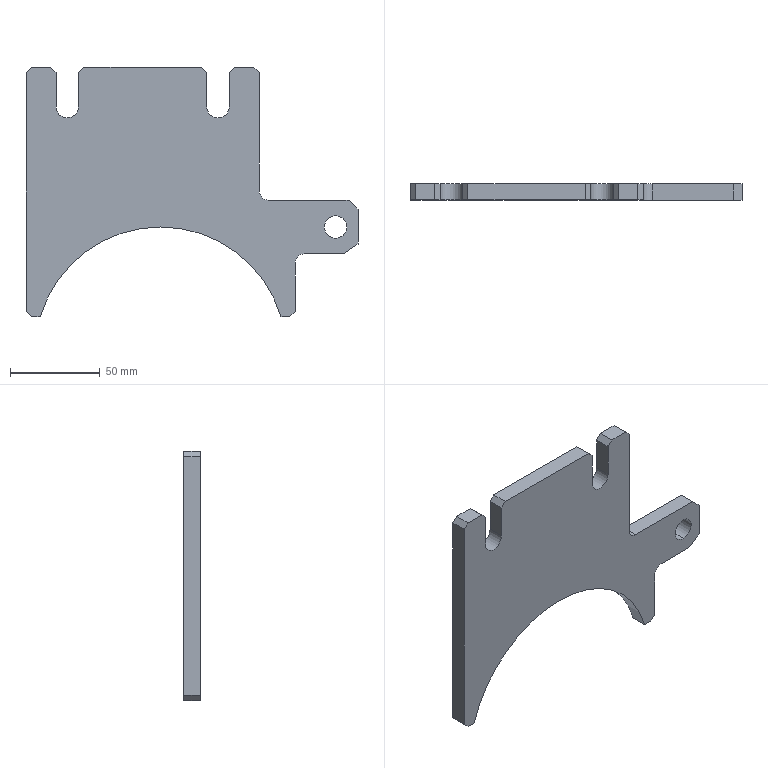Part | SolidWorks | features FlatPattern 1, SMBaseFlange 1, SheetMetal 1 | 1 solid | 35 faces | box 185 x 9 x 139 mm | volume 131664 mm3 | plane 27 | cylinder 8 | commonest cylinder face diameters 12.5 x4 10 x2 140 x2
STEP:
#1=CARTESIAN_POINT('',(172.5,-9.,43.75));
#2=VERTEX_POINT('',#1);
#3=CARTESIAN_POINT('',(172.5,-9.,56.25));
#4=VERTEX_POINT('',#3);
#5=CARTESIAN_POINT('',(172.5,-9.,50.));
#6=DIRECTION('',(0.,1.,0.));
#7=DIRECTION('',(0.,0.,1.));
#8=AXIS2_PLACEMENT_3D('',#5,#6,#7);
#9=CIRCLE('',#8,6.25);
#10=EDGE_CURVE('',#2,#4,#9,.T.);
#11=ORIENTED_EDGE('',*,*,#10,.F.);
#12=CARTESIAN_POINT('',(172.5,0.,43.75));
#13=VERTEX_POINT('',#12);
#14=CARTESIAN_POINT('',(172.5,-9.,43.75));
#15=DIRECTION('',(0.,1.,0.));
#16=VECTOR('',#15,1000.);
#17=LINE('',#14,#16);
#18=EDGE_CURVE('',#2,#13,#17,.T.);
#19=ORIENTED_EDGE('',*,*,#18,.T.);
#20=CARTESIAN_POINT('',(172.5,0.,56.25));
#21=VERTEX_POINT('',#20);
#22=CARTESIAN_POINT('',(172.5,0.,50.));
#23=DIRECTION('',(0.,1.,0.));
#24=DIRECTION('',(0.,0.,1.));
#25=AXIS2_PLACEMENT_3D('',#22,#23,#24);
#26=CIRCLE('',#25,6.25);
#27=EDGE_CURVE('',#13,#21,#26,.T.);
#28=ORIENTED_EDGE('',*,*,#27,.T.);
#29=CARTESIAN_POINT('',(172.5,-9.,56.25));
#30=DIRECTION('',(0.,1.,0.));
#31=VECTOR('',#30,1000.);
#32=LINE('',#29,#31);
#33=EDGE_CURVE('',#4,#21,#32,.T.);
#34=ORIENTED_EDGE('',*,*,#33,.F.);
#35=EDGE_LOOP('',(#11,#19,#28,#34));
#36=FACE_OUTER_BOUND('',#35,.T.);
#37=CARTESIAN_POINT('',(172.5,-9.,50.));
#38=DIRECTION('',(0.,1.,0.));
#39=DIRECTION('',(0.,0.,1.));
#40=AXIS2_PLACEMENT_3D('',#37,#38,#39);
#41=CYLINDRICAL_SURFACE('',#40,6.25);
#42=ADVANCED_FACE('',(#36),#41,.F.);
#43=CARTESIAN_POINT('',(142.082,-9.,0.));
#44=VERTEX_POINT('',#43);
#45=CARTESIAN_POINT('',(75.,-9.,50.));
#46=VERTEX_POINT('',#45);
#47=CARTESIAN_POINT('',(75.,-9.,-20.));
#48=DIRECTION('',(0.,-1.,0.));
#49=DIRECTION('',(0.,0.,1.));
#50=AXIS2_PLACEMENT_3D('',#47,#48,#49);
#51=CIRCLE('',#50,70.);
#52=EDGE_CURVE('',#44,#46,#51,.T.);
#53=ORIENTED_EDGE('',*,*,#52,.T.);
#54=CARTESIAN_POINT('',(75.,0.,50.));
#55=VERTEX_POINT('',#54);
#56=CARTESIAN_POINT('',(75.,-9.,50.));
#57=DIRECTION('',(0.,1.,0.));
#58=VECTOR('',#57,1000.);
#59=LINE('',#56,#58);
#60=EDGE_CURVE('',#46,#55,#59,.T.);
#61=ORIENTED_EDGE('',*,*,#60,.T.);
#62=CARTESIAN_POINT('',(142.082,0.,0.));
#63=VERTEX_POINT('',#62);
#64=CARTESIAN_POINT('',(75.,0.,-20.));
#65=DIRECTION('',(0.,-1.,0.));
#66=DIRECTION('',(0.,0.,1.));
#67=AXIS2_PLACEMENT_3D('',#64,#65,#66);
#68=CIRCLE('',#67,70.);
#69=EDGE_CURVE('',#63,#55,#68,.T.);
#70=ORIENTED_EDGE('',*,*,#69,.F.);
#71=CARTESIAN_POINT('',(142.082,-9.,0.));
#72=DIRECTION('',(0.,1.,0.));
#73=VECTOR('',#72,1000.);
#74=LINE('',#71,#73);
#75=EDGE_CURVE('',#44,#63,#74,.T.);
#76=ORIENTED_EDGE('',*,*,#75,.F.);
#77=EDGE_LOOP('',(#53,#61,#70,#76));
#78=FACE_OUTER_BOUND('',#77,.T.);
#79=CARTESIAN_POINT('',(75.,-9.,-20.));
#80=DIRECTION('',(0.,1.,0.));
#81=DIRECTION('',(0.,0.,1.));
#82=AXIS2_PLACEMENT_3D('',#79,#80,#81);
#83=CYLINDRICAL_SURFACE('',#82,70.);
#84=ADVANCED_FACE('',(#78),#83,.F.);
#85=ORIENTED_EDGE('',*,*,#60,.F.);
#86=CARTESIAN_POINT('',(7.918,-9.,0.));
#87=VERTEX_POINT('',#86);
#88=CARTESIAN_POINT('',(75.,-9.,-20.));
#89=DIRECTION('',(0.,-1.,0.));
#90=DIRECTION('',(0.,0.,1.));
#91=AXIS2_PLACEMENT_3D('',#88,#89,#90);
#92=CIRCLE('',#91,70.);
#93=EDGE_CURVE('',#46,#87,#92,.T.);
#94=ORIENTED_EDGE('',*,*,#93,.T.);
#95=CARTESIAN_POINT('',(7.918,0.,0.));
#96=VERTEX_POINT('',#95);
#97=CARTESIAN_POINT('',(7.918,-9.,0.));
#98=DIRECTION('',(0.,1.,0.));
#99=VECTOR('',#98,1000.);
#100=LINE('',#97,#99);
#101=EDGE_CURVE('',#87,#96,#100,.T.);
#102=ORIENTED_EDGE('',*,*,#101,.T.);
#103=CARTESIAN_POINT('',(75.,0.,-20.));
#104=DIRECTION('',(0.,-1.,0.));
#105=DIRECTION('',(0.,0.,1.));
#106=AXIS2_PLACEMENT_3D('',#103,#104,#105);
#107=CIRCLE('',#106,70.);
#108=EDGE_CURVE('',#55,#96,#107,.T.);
#109=ORIENTED_EDGE('',*,*,#108,.F.);
#110=EDGE_LOOP('',(#85,#94,#102,#109));
#111=FACE_OUTER_BOUND('',#110,.T.);
#112=CARTESIAN_POINT('',(75.,-9.,-20.));
#113=DIRECTION('',(0.,1.,0.));
#114=DIRECTION('',(0.,0.,1.));
#115=AXIS2_PLACEMENT_3D('',#112,#113,#114);
#116=CYLINDRICAL_SURFACE('',#115,70.);
#117=ADVANCED_FACE('',(#111),#116,.F.);
#118=CARTESIAN_POINT('',(147.,0.,0.));
#119=VERTEX_POINT('',#118);
#120=CARTESIAN_POINT('',(142.082,0.,0.));
#121=DIRECTION('',(-1.,0.,0.));
#122=VECTOR('',#121,1000.);
#123=LINE('',#120,#122);
#124=EDGE_CURVE('',#119,#63,#123,.T.);
#125=ORIENTED_EDGE('',*,*,#124,.F.);
#126=CARTESIAN_POINT('',(147.,-9.,0.));
#127=VERTEX_POINT('',#126);
#128=CARTESIAN_POINT('',(147.,-9.,0.));
#129=DIRECTION('',(0.,1.,0.));
#130=VECTOR('',#129,1000.);
#131=LINE('',#128,#130);
#132=EDGE_CURVE('',#127,#119,#131,.T.);
#133=ORIENTED_EDGE('',*,*,#132,.F.);
#134=CARTESIAN_POINT('',(142.082,-9.,0.));
#135=DIRECTION('',(-1.,0.,0.));
#136=VECTOR('',#135,1000.);
#137=LINE('',#134,#136);
#138=EDGE_CURVE('',#127,#44,#137,.T.);
#139=ORIENTED_EDGE('',*,*,#138,.T.);
#140=ORIENTED_EDGE('',*,*,#75,.T.);
#141=EDGE_LOOP('',(#125,#133,#139,#140));
#142=FACE_OUTER_BOUND('',#141,.T.);
#143=CARTESIAN_POINT('',(142.082,-9.,0.));
#144=DIRECTION('',(0.,0.,-1.));
#145=DIRECTION('',(-1.,0.,0.));
#146=AXIS2_PLACEMENT_3D('',#143,#144,#145);
#147=PLANE('',#146);
#148=ADVANCED_FACE('',(#142),#147,.T.);
#149=CARTESIAN_POINT('',(150.,0.,3.));
#150=VERTEX_POINT('',#149);
#151=CARTESIAN_POINT('',(147.,0.,0.));
#152=DIRECTION('',(-0.7071,0.,-0.7071));
#153=VECTOR('',#152,1000.);
#154=LINE('',#151,#153);
#155=EDGE_CURVE('',#150,#119,#154,.T.);
#156=ORIENTED_EDGE('',*,*,#155,.F.);
#157=CARTESIAN_POINT('',(150.,-9.,3.));
#158=VERTEX_POINT('',#157);
#159=CARTESIAN_POINT('',(150.,-9.,3.));
#160=DIRECTION('',(0.,1.,0.));
#161=VECTOR('',#160,1000.);
#162=LINE('',#159,#161);
#163=EDGE_CURVE('',#158,#150,#162,.T.);
#164=ORIENTED_EDGE('',*,*,#163,.F.);
#165=CARTESIAN_POINT('',(147.,-9.,0.));
#166=DIRECTION('',(-0.7071,0.,-0.7071));
#167=VECTOR('',#166,1000.);
#168=LINE('',#165,#167);
#169=EDGE_CURVE('',#158,#127,#168,.T.);
#170=ORIENTED_EDGE('',*,*,#169,.T.);
#171=ORIENTED_EDGE('',*,*,#132,.T.);
#172=EDGE_LOOP('',(#156,#164,#170,#171));
#173=FACE_OUTER_BOUND('',#172,.T.);
#174=CARTESIAN_POINT('',(147.,-9.,0.));
#175=DIRECTION('',(0.7071,0.,-0.7071));
#176=DIRECTION('',(-0.7071,0.,-0.7071));
#177=AXIS2_PLACEMENT_3D('',#174,#175,#176);
#178=PLANE('',#177);
#179=ADVANCED_FACE('',(#173),#178,.T.);
#180=CARTESIAN_POINT('',(150.,0.,30.));
#181=VERTEX_POINT('',#180);
#182=CARTESIAN_POINT('',(150.,0.,3.));
#183=DIRECTION('',(0.,0.,-1.));
#184=VECTOR('',#183,1000.);
#185=LINE('',#182,#184);
#186=EDGE_CURVE('',#181,#150,#185,.T.);
#187=ORIENTED_EDGE('',*,*,#186,.F.);
#188=CARTESIAN_POINT('',(150.,-9.,30.));
#189=VERTEX_POINT('',#188);
#190=CARTESIAN_POINT('',(150.,-9.,30.));
#191=DIRECTION('',(0.,1.,0.));
#192=VECTOR('',#191,1000.);
#193=LINE('',#190,#192);
#194=EDGE_CURVE('',#189,#181,#193,.T.);
#195=ORIENTED_EDGE('',*,*,#194,.F.);
#196=CARTESIAN_POINT('',(150.,-9.,3.));
#197=DIRECTION('',(0.,0.,-1.));
#198=VECTOR('',#197,1000.);
#199=LINE('',#196,#198);
#200=EDGE_CURVE('',#189,#158,#199,.T.);
#201=ORIENTED_EDGE('',*,*,#200,.T.);
#202=ORIENTED_EDGE('',*,*,#163,.T.);
#203=EDGE_LOOP('',(#187,#195,#201,#202));
#204=FACE_OUTER_BOUND('',#203,.T.);
#205=CARTESIAN_POINT('',(150.,-9.,3.));
#206=DIRECTION('',(1.,0.,0.));
#207=DIRECTION('',(0.,0.,-1.));
#208=AXIS2_PLACEMENT_3D('',#205,#206,#207);
#209=PLANE('',#208);
#210=ADVANCED_FACE('',(#204),#209,.T.);
#211=CARTESIAN_POINT('',(155.,0.,35.));
#212=VERTEX_POINT('',#211);
#213=CARTESIAN_POINT('',(155.,0.,30.));
#214=DIRECTION('',(0.,-1.,0.));
#215=DIRECTION('',(0.,0.,1.));
#216=AXIS2_PLACEMENT_3D('',#213,#214,#215);
#217=CIRCLE('',#216,5.);
#218=EDGE_CURVE('',#212,#181,#217,.T.);
#219=ORIENTED_EDGE('',*,*,#218,.F.);
#220=CARTESIAN_POINT('',(155.,-9.,35.));
#221=VERTEX_POINT('',#220);
#222=CARTESIAN_POINT('',(155.,-9.,35.));
#223=DIRECTION('',(0.,1.,0.));
#224=VECTOR('',#223,1000.);
#225=LINE('',#222,#224);
#226=EDGE_CURVE('',#221,#212,#225,.T.);
#227=ORIENTED_EDGE('',*,*,#226,.F.);
#228=CARTESIAN_POINT('',(155.,-9.,30.));
#229=DIRECTION('',(0.,-1.,0.));
#230=DIRECTION('',(0.,0.,1.));
#231=AXIS2_PLACEMENT_3D('',#228,#229,#230);
#232=CIRCLE('',#231,5.);
#233=EDGE_CURVE('',#221,#189,#232,.T.);
#234=ORIENTED_EDGE('',*,*,#233,.T.);
#235=ORIENTED_EDGE('',*,*,#194,.T.);
#236=EDGE_LOOP('',(#219,#227,#234,#235));
#237=FACE_OUTER_BOUND('',#236,.T.);
#238=CARTESIAN_POINT('',(155.,-9.,30.));
#239=DIRECTION('',(0.,1.,0.));
#240=DIRECTION('',(0.,0.,1.));
#241=AXIS2_PLACEMENT_3D('',#238,#239,#240);
#242=CYLINDRICAL_SURFACE('',#241,5.);
#243=ADVANCED_FACE('',(#237),#242,.F.);
#244=CARTESIAN_POINT('',(177.,0.,35.));
#245=VERTEX_POINT('',#244);
#246=CARTESIAN_POINT('',(155.,0.,35.));
#247=DIRECTION('',(-1.,0.,0.));
#248=VECTOR('',#247,1000.);
#249=LINE('',#246,#248);
#250=EDGE_CURVE('',#245,#212,#249,.T.);
#251=ORIENTED_EDGE('',*,*,#250,.F.);
#252=CARTESIAN_POINT('',(177.,-9.,35.));
#253=VERTEX_POINT('',#252);
#254=CARTESIAN_POINT('',(177.,-9.,35.));
#255=DIRECTION('',(0.,1.,0.));
#256=VECTOR('',#255,1000.);
#257=LINE('',#254,#256);
#258=EDGE_CURVE('',#253,#245,#257,.T.);
#259=ORIENTED_EDGE('',*,*,#258,.F.);
#260=CARTESIAN_POINT('',(155.,-9.,35.));
#261=DIRECTION('',(-1.,0.,0.));
#262=VECTOR('',#261,1000.);
#263=LINE('',#260,#262);
#264=EDGE_CURVE('',#253,#221,#263,.T.);
#265=ORIENTED_EDGE('',*,*,#264,.T.);
#266=ORIENTED_EDGE('',*,*,#226,.T.);
#267=EDGE_LOOP('',(#251,#259,#265,#266));
#268=FACE_OUTER_BOUND('',#267,.T.);
#269=CARTESIAN_POINT('',(155.,-9.,35.));
#270=DIRECTION('',(0.,0.,-1.));
#271=DIRECTION('',(-1.,0.,0.));
#272=AXIS2_PLACEMENT_3D('',#269,#270,#271);
#273=PLANE('',#272);
#274=ADVANCED_FACE('',(#268),#273,.T.);
#275=CARTESIAN_POINT('',(185.,0.,40.5));
#276=VERTEX_POINT('',#275);
#277=CARTESIAN_POINT('',(185.,0.,40.5));
#278=DIRECTION('',(-0.824,0.,-0.5665));
#279=VECTOR('',#278,1000.);
#280=LINE('',#277,#279);
#281=EDGE_CURVE('',#276,#245,#280,.T.);
#282=ORIENTED_EDGE('',*,*,#281,.F.);
#283=CARTESIAN_POINT('',(185.,-9.,40.5));
#284=VERTEX_POINT('',#283);
#285=CARTESIAN_POINT('',(185.,-9.,40.5));
#286=DIRECTION('',(0.,1.,0.));
#287=VECTOR('',#286,1000.);
#288=LINE('',#285,#287);
#289=EDGE_CURVE('',#284,#276,#288,.T.);
#290=ORIENTED_EDGE('',*,*,#289,.F.);
#291=CARTESIAN_POINT('',(185.,-9.,40.5));
#292=DIRECTION('',(-0.824,0.,-0.5665));
#293=VECTOR('',#292,1000.);
#294=LINE('',#291,#293);
#295=EDGE_CURVE('',#284,#253,#294,.T.);
#296=ORIENTED_EDGE('',*,*,#295,.T.);
#297=ORIENTED_EDGE('',*,*,#258,.T.);
#298=EDGE_LOOP('',(#282,#290,#296,#297));
#299=FACE_OUTER_BOUND('',#298,.T.);
#300=CARTESIAN_POINT('',(185.,-9.,40.5));
#301=DIRECTION('',(0.5665,0.,-0.824));
#302=DIRECTION('',(-0.824,0.,-0.5665));
#303=AXIS2_PLACEMENT_3D('',#300,#301,#302);
#304=PLANE('',#303);
#305=ADVANCED_FACE('',(#299),#304,.T.);
#306=CARTESIAN_POINT('',(185.,0.,60.));
#307=VERTEX_POINT('',#306);
#308=CARTESIAN_POINT('',(185.,0.,40.5));
#309=DIRECTION('',(0.,0.,-1.));
#310=VECTOR('',#309,1000.);
#311=LINE('',#308,#310);
#312=EDGE_CURVE('',#307,#276,#311,.T.);
#313=ORIENTED_EDGE('',*,*,#312,.F.);
#314=CARTESIAN_POINT('',(185.,-9.,60.));
#315=VERTEX_POINT('',#314);
#316=CARTESIAN_POINT('',(185.,-9.,60.));
#317=DIRECTION('',(0.,1.,0.));
#318=VECTOR('',#317,1000.);
#319=LINE('',#316,#318);
#320=EDGE_CURVE('',#315,#307,#319,.T.);
#321=ORIENTED_EDGE('',*,*,#320,.F.);
#322=CARTESIAN_POINT('',(185.,-9.,40.5));
#323=DIRECTION('',(0.,0.,-1.));
#324=VECTOR('',#323,1000.);
#325=LINE('',#322,#324);
#326=EDGE_CURVE('',#315,#284,#325,.T.);
#327=ORIENTED_EDGE('',*,*,#326,.T.);
#328=ORIENTED_EDGE('',*,*,#289,.T.);
#329=EDGE_LOOP('',(#313,#321,#327,#328));
#330=FACE_OUTER_BOUND('',#329,.T.);
#331=CARTESIAN_POINT('',(185.,-9.,40.5));
#332=DIRECTION('',(1.,0.,0.));
#333=DIRECTION('',(0.,0.,-1.));
#334=AXIS2_PLACEMENT_3D('',#331,#332,#333);
#335=PLANE('',#334);
#336=ADVANCED_FACE('',(#330),#335,.T.);
#337=CARTESIAN_POINT('',(180.,0.,65.));
#338=VERTEX_POINT('',#337);
#339=CARTESIAN_POINT('',(185.,0.,60.));
#340=DIRECTION('',(0.7071,0.,-0.7071));
#341=VECTOR('',#340,1000.);
#342=LINE('',#339,#341);
#343=EDGE_CURVE('',#338,#307,#342,.T.);
#344=ORIENTED_EDGE('',*,*,#343,.F.);
#345=CARTESIAN_POINT('',(180.,-9.,65.));
#346=VERTEX_POINT('',#345);
#347=CARTESIAN_POINT('',(180.,-9.,65.));
#348=DIRECTION('',(0.,1.,0.));
#349=VECTOR('',#348,1000.);
#350=LINE('',#347,#349);
#351=EDGE_CURVE('',#346,#338,#350,.T.);
#352=ORIENTED_EDGE('',*,*,#351,.F.);
#353=CARTESIAN_POINT('',(185.,-9.,60.));
#354=DIRECTION('',(0.7071,0.,-0.7071));
#355=VECTOR('',#354,1000.);
#356=LINE('',#353,#355);
#357=EDGE_CURVE('',#346,#315,#356,.T.);
#358=ORIENTED_EDGE('',*,*,#357,.T.);
#359=ORIENTED_EDGE('',*,*,#320,.T.);
#360=EDGE_LOOP('',(#344,#352,#358,#359));
#361=FACE_OUTER_BOUND('',#360,.T.);
#362=CARTESIAN_POINT('',(185.,-9.,60.));
#363=DIRECTION('',(0.7071,0.,0.7071));
#364=DIRECTION('',(0.7071,0.,-0.7071));
#365=AXIS2_PLACEMENT_3D('',#362,#363,#364);
#366=PLANE('',#365);
#367=ADVANCED_FACE('',(#361),#366,.T.);
#368=CARTESIAN_POINT('',(135.,0.,65.));
#369=VERTEX_POINT('',#368);
#370=CARTESIAN_POINT('',(180.,0.,65.));
#371=DIRECTION('',(1.,0.,0.));
#372=VECTOR('',#371,1000.);
#373=LINE('',#370,#372);
#374=EDGE_CURVE('',#369,#338,#373,.T.);
#375=ORIENTED_EDGE('',*,*,#374,.F.);
#376=CARTESIAN_POINT('',(135.,-9.,65.));
#377=VERTEX_POINT('',#376);
#378=CARTESIAN_POINT('',(135.,-9.,65.));
#379=DIRECTION('',(0.,1.,0.));
#380=VECTOR('',#379,1000.);
#381=LINE('',#378,#380);
#382=EDGE_CURVE('',#377,#369,#381,.T.);
#383=ORIENTED_EDGE('',*,*,#382,.F.);
#384=CARTESIAN_POINT('',(180.,-9.,65.));
#385=DIRECTION('',(1.,0.,0.));
#386=VECTOR('',#385,1000.);
#387=LINE('',#384,#386);
#388=EDGE_CURVE('',#377,#346,#387,.T.);
#389=ORIENTED_EDGE('',*,*,#388,.T.);
#390=ORIENTED_EDGE('',*,*,#351,.T.);
#391=EDGE_LOOP('',(#375,#383,#389,#390));
#392=FACE_OUTER_BOUND('',#391,.T.);
#393=CARTESIAN_POINT('',(180.,-9.,65.));
#394=DIRECTION('',(0.,0.,1.));
#395=DIRECTION('',(1.,0.,0.));
#396=AXIS2_PLACEMENT_3D('',#393,#394,#395);
#397=PLANE('',#396);
#398=ADVANCED_FACE('',(#392),#397,.T.);
#399=CARTESIAN_POINT('',(130.,0.,70.));
#400=VERTEX_POINT('',#399);
#401=CARTESIAN_POINT('',(135.,0.,70.));
#402=DIRECTION('',(0.,-1.,0.));
#403=DIRECTION('',(0.,0.,1.));
#404=AXIS2_PLACEMENT_3D('',#401,#402,#403);
#405=CIRCLE('',#404,5.);
#406=EDGE_CURVE('',#400,#369,#405,.T.);
#407=ORIENTED_EDGE('',*,*,#406,.F.);
#408=CARTESIAN_POINT('',(130.,-9.,70.));
#409=VERTEX_POINT('',#408);
#410=CARTESIAN_POINT('',(130.,-9.,70.));
#411=DIRECTION('',(0.,1.,0.));
#412=VECTOR('',#411,1000.);
#413=LINE('',#410,#412);
#414=EDGE_CURVE('',#409,#400,#413,.T.);
#415=ORIENTED_EDGE('',*,*,#414,.F.);
#416=CARTESIAN_POINT('',(135.,-9.,70.));
#417=DIRECTION('',(0.,-1.,0.));
#418=DIRECTION('',(0.,0.,1.));
#419=AXIS2_PLACEMENT_3D('',#416,#417,#418);
#420=CIRCLE('',#419,5.);
#421=EDGE_CURVE('',#409,#377,#420,.T.);
#422=ORIENTED_EDGE('',*,*,#421,.T.);
#423=ORIENTED_EDGE('',*,*,#382,.T.);
#424=EDGE_LOOP('',(#407,#415,#422,#423));
#425=FACE_OUTER_BOUND('',#424,.T.);
#426=CARTESIAN_POINT('',(135.,-9.,70.));
#427=DIRECTION('',(0.,1.,0.));
#428=DIRECTION('',(0.,0.,1.));
#429=AXIS2_PLACEMENT_3D('',#426,#427,#428);
#430=CYLINDRICAL_SURFACE('',#429,5.);
#431=ADVANCED_FACE('',(#425),#430,.F.);
#432=CARTESIAN_POINT('',(130.,0.,136.));
#433=VERTEX_POINT('',#432);
#434=CARTESIAN_POINT('',(130.,0.,70.));
#435=DIRECTION('',(0.,0.,-1.));
#436=VECTOR('',#435,1000.);
#437=LINE('',#434,#436);
#438=EDGE_CURVE('',#433,#400,#437,.T.);
#439=ORIENTED_EDGE('',*,*,#438,.F.);
#440=CARTESIAN_POINT('',(130.,-9.,136.));
#441=VERTEX_POINT('',#440);
#442=CARTESIAN_POINT('',(130.,-9.,136.));
#443=DIRECTION('',(0.,1.,0.));
#444=VECTOR('',#443,1000.);
#445=LINE('',#442,#444);
#446=EDGE_CURVE('',#441,#433,#445,.T.);
#447=ORIENTED_EDGE('',*,*,#446,.F.);
#448=CARTESIAN_POINT('',(130.,-9.,70.));
#449=DIRECTION('',(0.,0.,-1.));
#450=VECTOR('',#449,1000.);
#451=LINE('',#448,#450);
#452=EDGE_CURVE('',#441,#409,#451,.T.);
#453=ORIENTED_EDGE('',*,*,#452,.T.);
#454=ORIENTED_EDGE('',*,*,#414,.T.);
#455=EDGE_LOOP('',(#439,#447,#453,#454));
#456=FACE_OUTER_BOUND('',#455,.T.);
#457=CARTESIAN_POINT('',(130.,-9.,70.));
#458=DIRECTION('',(1.,0.,0.));
#459=DIRECTION('',(0.,0.,-1.));
#460=AXIS2_PLACEMENT_3D('',#457,#458,#459);
#461=PLANE('',#460);
#462=ADVANCED_FACE('',(#456),#461,.T.);
#463=CARTESIAN_POINT('',(127.,0.,139.));
#464=VERTEX_POINT('',#463);
#465=CARTESIAN_POINT('',(130.,0.,136.));
#466=DIRECTION('',(0.7071,0.,-0.7071));
#467=VECTOR('',#466,1000.);
#468=LINE('',#465,#467);
#469=EDGE_CURVE('',#464,#433,#468,.T.);
#470=ORIENTED_EDGE('',*,*,#469,.F.);
#471=CARTESIAN_POINT('',(127.,-9.,139.));
#472=VERTEX_POINT('',#471);
#473=CARTESIAN_POINT('',(127.,-9.,139.));
#474=DIRECTION('',(0.,1.,0.));
#475=VECTOR('',#474,1000.);
#476=LINE('',#473,#475);
#477=EDGE_CURVE('',#472,#464,#476,.T.);
#478=ORIENTED_EDGE('',*,*,#477,.F.);
#479=CARTESIAN_POINT('',(130.,-9.,136.));
#480=DIRECTION('',(0.7071,0.,-0.7071));
#481=VECTOR('',#480,1000.);
#482=LINE('',#479,#481);
#483=EDGE_CURVE('',#472,#441,#482,.T.);
#484=ORIENTED_EDGE('',*,*,#483,.T.);
#485=ORIENTED_EDGE('',*,*,#446,.T.);
#486=EDGE_LOOP('',(#470,#478,#484,#485));
#487=FACE_OUTER_BOUND('',#486,.T.);
#488=CARTESIAN_POINT('',(130.,-9.,136.));
#489=DIRECTION('',(0.7071,0.,0.7071));
#490=DIRECTION('',(0.7071,0.,-0.7071));
#491=AXIS2_PLACEMENT_3D('',#488,#489,#490);
#492=PLANE('',#491);
#493=ADVANCED_FACE('',(#487),#492,.T.);
#494=CARTESIAN_POINT('',(116.25,0.,139.));
#495=VERTEX_POINT('',#494);
#496=CARTESIAN_POINT('',(116.25,0.,139.));
#497=DIRECTION('',(1.,0.,0.));
#498=VECTOR('',#497,1000.);
#499=LINE('',#496,#498);
#500=EDGE_CURVE('',#495,#464,#499,.T.);
#501=ORIENTED_EDGE('',*,*,#500,.F.);
#502=CARTESIAN_POINT('',(116.25,-9.,139.));
#503=VERTEX_POINT('',#502);
#504=CARTESIAN_POINT('',(116.25,-9.,139.));
#505=DIRECTION('',(0.,1.,0.));
#506=VECTOR('',#505,1000.);
#507=LINE('',#504,#506);
#508=EDGE_CURVE('',#503,#495,#507,.T.);
#509=ORIENTED_EDGE('',*,*,#508,.F.);
#510=CARTESIAN_POINT('',(116.25,-9.,139.));
#511=DIRECTION('',(1.,0.,0.));
#512=VECTOR('',#511,1000.);
#513=LINE('',#510,#512);
#514=EDGE_CURVE('',#503,#472,#513,.T.);
#515=ORIENTED_EDGE('',*,*,#514,.T.);
#516=ORIENTED_EDGE('',*,*,#477,.T.);
#517=EDGE_LOOP('',(#501,#509,#515,#516));
#518=FACE_OUTER_BOUND('',#517,.T.);
#519=CARTESIAN_POINT('',(116.25,-9.,139.));
#520=DIRECTION('',(0.,0.,1.));
#521=DIRECTION('',(1.,0.,0.));
#522=AXIS2_PLACEMENT_3D('',#519,#520,#521);
#523=PLANE('',#522);
#524=ADVANCED_FACE('',(#518),#523,.T.);
#525=CARTESIAN_POINT('',(113.25,0.,136.));
#526=VERTEX_POINT('',#525);
#527=CARTESIAN_POINT('',(113.25,0.,136.));
#528=DIRECTION('',(0.7071,0.,0.7071));
#529=VECTOR('',#528,1000.);
#530=LINE('',#527,#529);
#531=EDGE_CURVE('',#526,#495,#530,.T.);
#532=ORIENTED_EDGE('',*,*,#531,.F.);
#533=CARTESIAN_POINT('',(113.25,-9.,136.));
#534=VERTEX_POINT('',#533);
#535=CARTESIAN_POINT('',(113.25,-9.,136.));
#536=DIRECTION('',(0.,1.,0.));
#537=VECTOR('',#536,1000.);
#538=LINE('',#535,#537);
#539=EDGE_CURVE('',#534,#526,#538,.T.);
#540=ORIENTED_EDGE('',*,*,#539,.F.);
#541=CARTESIAN_POINT('',(113.25,-9.,136.));
#542=DIRECTION('',(0.7071,0.,0.7071));
#543=VECTOR('',#542,1000.);
#544=LINE('',#541,#543);
#545=EDGE_CURVE('',#534,#503,#544,.T.);
#546=ORIENTED_EDGE('',*,*,#545,.T.);
#547=ORIENTED_EDGE('',*,*,#508,.T.);
#548=EDGE_LOOP('',(#532,#540,#546,#547));
#549=FACE_OUTER_BOUND('',#548,.T.);
#550=CARTESIAN_POINT('',(113.25,-9.,136.));
#551=DIRECTION('',(-0.7071,0.,0.7071));
#552=DIRECTION('',(0.7071,0.,0.7071));
#553=AXIS2_PLACEMENT_3D('',#550,#551,#552);
#554=PLANE('',#553);
#555=ADVANCED_FACE('',(#549),#554,.T.);
#556=CARTESIAN_POINT('',(113.25,0.,117.));
#557=VERTEX_POINT('',#556);
#558=CARTESIAN_POINT('',(113.25,0.,117.));
#559=DIRECTION('',(0.,0.,1.));
#560=VECTOR('',#559,1000.);
#561=LINE('',#558,#560);
#562=EDGE_CURVE('',#557,#526,#561,.T.);
#563=ORIENTED_EDGE('',*,*,#562,.F.);
#564=CARTESIAN_POINT('',(113.25,-9.,117.));
#565=VERTEX_POINT('',#564);
#566=CARTESIAN_POINT('',(113.25,-9.,117.));
#567=DIRECTION('',(0.,1.,0.));
#568=VECTOR('',#567,1000.);
#569=LINE('',#566,#568);
#570=EDGE_CURVE('',#565,#557,#569,.T.);
#571=ORIENTED_EDGE('',*,*,#570,.F.);
#572=CARTESIAN_POINT('',(113.25,-9.,117.));
#573=DIRECTION('',(0.,0.,1.));
#574=VECTOR('',#573,1000.);
#575=LINE('',#572,#574);
#576=EDGE_CURVE('',#565,#534,#575,.T.);
#577=ORIENTED_EDGE('',*,*,#576,.T.);
#578=ORIENTED_EDGE('',*,*,#539,.T.);
#579=EDGE_LOOP('',(#563,#571,#577,#578));
#580=FACE_OUTER_BOUND('',#579,.T.);
#581=CARTESIAN_POINT('',(113.25,-9.,117.));
#582=DIRECTION('',(-1.,0.,0.));
#583=DIRECTION('',(0.,0.,1.));
#584=AXIS2_PLACEMENT_3D('',#581,#582,#583);
#585=PLANE('',#584);
#586=ADVANCED_FACE('',(#580),#585,.T.);
#587=CARTESIAN_POINT('',(100.75,0.,117.));
#588=VERTEX_POINT('',#587);
#589=CARTESIAN_POINT('',(107.,0.,117.));
#590=DIRECTION('',(0.,-1.,0.));
#591=DIRECTION('',(0.,0.,1.));
#592=AXIS2_PLACEMENT_3D('',#589,#590,#591);
#593=CIRCLE('',#592,6.25);
#594=EDGE_CURVE('',#588,#557,#593,.T.);
#595=ORIENTED_EDGE('',*,*,#594,.F.);
#596=CARTESIAN_POINT('',(100.75,-9.,117.));
#597=VERTEX_POINT('',#596);
#598=CARTESIAN_POINT('',(100.75,-9.,117.));
#599=DIRECTION('',(0.,1.,0.));
#600=VECTOR('',#599,1000.);
#601=LINE('',#598,#600);
#602=EDGE_CURVE('',#597,#588,#601,.T.);
#603=ORIENTED_EDGE('',*,*,#602,.F.);
#604=CARTESIAN_POINT('',(107.,-9.,117.));
#605=DIRECTION('',(0.,-1.,0.));
#606=DIRECTION('',(0.,0.,1.));
#607=AXIS2_PLACEMENT_3D('',#604,#605,#606);
#608=CIRCLE('',#607,6.25);
#609=EDGE_CURVE('',#597,#565,#608,.T.);
#610=ORIENTED_EDGE('',*,*,#609,.T.);
#611=ORIENTED_EDGE('',*,*,#570,.T.);
#612=EDGE_LOOP('',(#595,#603,#610,#611));
#613=FACE_OUTER_BOUND('',#612,.T.);
#614=CARTESIAN_POINT('',(107.,-9.,117.));
#615=DIRECTION('',(0.,1.,0.));
#616=DIRECTION('',(0.,0.,1.));
#617=AXIS2_PLACEMENT_3D('',#614,#615,#616);
#618=CYLINDRICAL_SURFACE('',#617,6.25);
#619=ADVANCED_FACE('',(#613),#618,.F.);
#620=CARTESIAN_POINT('',(100.75,0.,136.));
#621=VERTEX_POINT('',#620);
#622=CARTESIAN_POINT('',(100.75,0.,117.));
#623=DIRECTION('',(0.,0.,-1.));
#624=VECTOR('',#623,1000.);
#625=LINE('',#622,#624);
#626=EDGE_CURVE('',#621,#588,#625,.T.);
#627=ORIENTED_EDGE('',*,*,#626,.F.);
#628=CARTESIAN_POINT('',(100.75,-9.,136.));
#629=VERTEX_POINT('',#628);
#630=CARTESIAN_POINT('',(100.75,-9.,136.));
#631=DIRECTION('',(0.,1.,0.));
#632=VECTOR('',#631,1000.);
#633=LINE('',#630,#632);
#634=EDGE_CURVE('',#629,#621,#633,.T.);
#635=ORIENTED_EDGE('',*,*,#634,.F.);
#636=CARTESIAN_POINT('',(100.75,-9.,117.));
#637=DIRECTION('',(0.,0.,-1.));
#638=VECTOR('',#637,1000.);
#639=LINE('',#636,#638);
#640=EDGE_CURVE('',#629,#597,#639,.T.);
#641=ORIENTED_EDGE('',*,*,#640,.T.);
#642=ORIENTED_EDGE('',*,*,#602,.T.);
#643=EDGE_LOOP('',(#627,#635,#641,#642));
#644=FACE_OUTER_BOUND('',#643,.T.);
#645=CARTESIAN_POINT('',(100.75,-9.,117.));
#646=DIRECTION('',(1.,0.,0.));
#647=DIRECTION('',(0.,0.,-1.));
#648=AXIS2_PLACEMENT_3D('',#645,#646,#647);
#649=PLANE('',#648);
#650=ADVANCED_FACE('',(#644),#649,.T.);
#651=CARTESIAN_POINT('',(97.75,0.,139.));
#652=VERTEX_POINT('',#651);
#653=CARTESIAN_POINT('',(100.75,0.,136.));
#654=DIRECTION('',(0.7071,0.,-0.7071));
#655=VECTOR('',#654,1000.);
#656=LINE('',#653,#655);
#657=EDGE_CURVE('',#652,#621,#656,.T.);
#658=ORIENTED_EDGE('',*,*,#657,.F.);
#659=CARTESIAN_POINT('',(97.75,-9.,139.));
#660=VERTEX_POINT('',#659);
#661=CARTESIAN_POINT('',(97.75,-9.,139.));
#662=DIRECTION('',(0.,1.,0.));
#663=VECTOR('',#662,1000.);
#664=LINE('',#661,#663);
#665=EDGE_CURVE('',#660,#652,#664,.T.);
#666=ORIENTED_EDGE('',*,*,#665,.F.);
#667=CARTESIAN_POINT('',(100.75,-9.,136.));
#668=DIRECTION('',(0.7071,0.,-0.7071));
#669=VECTOR('',#668,1000.);
#670=LINE('',#667,#669);
#671=EDGE_CURVE('',#660,#629,#670,.T.);
#672=ORIENTED_EDGE('',*,*,#671,.T.);
#673=ORIENTED_EDGE('',*,*,#634,.T.);
#674=EDGE_LOOP('',(#658,#666,#672,#673));
#675=FACE_OUTER_BOUND('',#674,.T.);
#676=CARTESIAN_POINT('',(100.75,-9.,136.));
#677=DIRECTION('',(0.7071,0.,0.7071));
#678=DIRECTION('',(0.7071,0.,-0.7071));
#679=AXIS2_PLACEMENT_3D('',#676,#677,#678);
#680=PLANE('',#679);
#681=ADVANCED_FACE('',(#675),#680,.T.);
#682=CARTESIAN_POINT('',(32.25,0.,139.));
#683=VERTEX_POINT('',#682);
#684=CARTESIAN_POINT('',(32.25,0.,139.));
#685=DIRECTION('',(1.,0.,0.));
#686=VECTOR('',#685,1000.);
#687=LINE('',#684,#686);
#688=EDGE_CURVE('',#683,#652,#687,.T.);
#689=ORIENTED_EDGE('',*,*,#688,.F.);
#690=CARTESIAN_POINT('',(32.25,-9.,139.));
#691=VERTEX_POINT('',#690);
#692=CARTESIAN_POINT('',(32.25,-9.,139.));
#693=DIRECTION('',(0.,1.,0.));
#694=VECTOR('',#693,1000.);
#695=LINE('',#692,#694);
#696=EDGE_CURVE('',#691,#683,#695,.T.);
#697=ORIENTED_EDGE('',*,*,#696,.F.);
#698=CARTESIAN_POINT('',(32.25,-9.,139.));
#699=DIRECTION('',(1.,0.,0.));
#700=VECTOR('',#699,1000.);
#701=LINE('',#698,#700);
#702=EDGE_CURVE('',#691,#660,#701,.T.);
#703=ORIENTED_EDGE('',*,*,#702,.T.);
#704=ORIENTED_EDGE('',*,*,#665,.T.);
#705=EDGE_LOOP('',(#689,#697,#703,#704));
#706=FACE_OUTER_BOUND('',#705,.T.);
#707=CARTESIAN_POINT('',(32.25,-9.,139.));
#708=DIRECTION('',(0.,0.,1.));
#709=DIRECTION('',(1.,0.,0.));
#710=AXIS2_PLACEMENT_3D('',#707,#708,#709);
#711=PLANE('',#710);
#712=ADVANCED_FACE('',(#706),#711,.T.);
#713=CARTESIAN_POINT('',(29.25,0.,136.));
#714=VERTEX_POINT('',#713);
#715=CARTESIAN_POINT('',(29.25,0.,136.));
#716=DIRECTION('',(0.7071,0.,0.7071));
#717=VECTOR('',#716,1000.);
#718=LINE('',#715,#717);
#719=EDGE_CURVE('',#714,#683,#718,.T.);
#720=ORIENTED_EDGE('',*,*,#719,.F.);
#721=CARTESIAN_POINT('',(29.25,-9.,136.));
#722=VERTEX_POINT('',#721);
#723=CARTESIAN_POINT('',(29.25,-9.,136.));
#724=DIRECTION('',(0.,1.,0.));
#725=VECTOR('',#724,1000.);
#726=LINE('',#723,#725);
#727=EDGE_CURVE('',#722,#714,#726,.T.);
#728=ORIENTED_EDGE('',*,*,#727,.F.);
#729=CARTESIAN_POINT('',(29.25,-9.,136.));
#730=DIRECTION('',(0.7071,0.,0.7071));
#731=VECTOR('',#730,1000.);
#732=LINE('',#729,#731);
#733=EDGE_CURVE('',#722,#691,#732,.T.);
#734=ORIENTED_EDGE('',*,*,#733,.T.);
#735=ORIENTED_EDGE('',*,*,#696,.T.);
#736=EDGE_LOOP('',(#720,#728,#734,#735));
#737=FACE_OUTER_BOUND('',#736,.T.);
#738=CARTESIAN_POINT('',(29.25,-9.,136.));
#739=DIRECTION('',(-0.7071,0.,0.7071));
#740=DIRECTION('',(0.7071,0.,0.7071));
#741=AXIS2_PLACEMENT_3D('',#738,#739,#740);
#742=PLANE('',#741);
#743=ADVANCED_FACE('',(#737),#742,.T.);
#744=CARTESIAN_POINT('',(29.25,0.,117.));
#745=VERTEX_POINT('',#744);
#746=CARTESIAN_POINT('',(29.25,0.,117.));
#747=DIRECTION('',(0.,0.,1.));
#748=VECTOR('',#747,1000.);
#749=LINE('',#746,#748);
#750=EDGE_CURVE('',#745,#714,#749,.T.);
#751=ORIENTED_EDGE('',*,*,#750,.F.);
#752=CARTESIAN_POINT('',(29.25,-9.,117.));
#753=VERTEX_POINT('',#752);
#754=CARTESIAN_POINT('',(29.25,-9.,117.));
#755=DIRECTION('',(0.,1.,0.));
#756=VECTOR('',#755,1000.);
#757=LINE('',#754,#756);
#758=EDGE_CURVE('',#753,#745,#757,.T.);
#759=ORIENTED_EDGE('',*,*,#758,.F.);
#760=CARTESIAN_POINT('',(29.25,-9.,117.));
#761=DIRECTION('',(0.,0.,1.));
#762=VECTOR('',#761,1000.);
#763=LINE('',#760,#762);
#764=EDGE_CURVE('',#753,#722,#763,.T.);
#765=ORIENTED_EDGE('',*,*,#764,.T.);
#766=ORIENTED_EDGE('',*,*,#727,.T.);
#767=EDGE_LOOP('',(#751,#759,#765,#766));
#768=FACE_OUTER_BOUND('',#767,.T.);
#769=CARTESIAN_POINT('',(29.25,-9.,117.));
#770=DIRECTION('',(-1.,0.,0.));
#771=DIRECTION('',(0.,0.,1.));
#772=AXIS2_PLACEMENT_3D('',#769,#770,#771);
#773=PLANE('',#772);
#774=ADVANCED_FACE('',(#768),#773,.T.);
#775=CARTESIAN_POINT('',(16.75,0.,117.));
#776=VERTEX_POINT('',#775);
#777=CARTESIAN_POINT('',(23.,0.,117.));
#778=DIRECTION('',(0.,-1.,0.));
#779=DIRECTION('',(0.,0.,1.));
#780=AXIS2_PLACEMENT_3D('',#777,#778,#779);
#781=CIRCLE('',#780,6.25);
#782=EDGE_CURVE('',#776,#745,#781,.T.);
#783=ORIENTED_EDGE('',*,*,#782,.F.);
#784=CARTESIAN_POINT('',(16.75,-9.,117.));
#785=VERTEX_POINT('',#784);
#786=CARTESIAN_POINT('',(16.75,-9.,117.));
#787=DIRECTION('',(0.,1.,0.));
#788=VECTOR('',#787,1000.);
#789=LINE('',#786,#788);
#790=EDGE_CURVE('',#785,#776,#789,.T.);
#791=ORIENTED_EDGE('',*,*,#790,.F.);
#792=CARTESIAN_POINT('',(23.,-9.,117.));
#793=DIRECTION('',(0.,-1.,0.));
#794=DIRECTION('',(0.,0.,1.));
#795=AXIS2_PLACEMENT_3D('',#792,#793,#794);
#796=CIRCLE('',#795,6.25);
#797=EDGE_CURVE('',#785,#753,#796,.T.);
#798=ORIENTED_EDGE('',*,*,#797,.T.);
#799=ORIENTED_EDGE('',*,*,#758,.T.);
#800=EDGE_LOOP('',(#783,#791,#798,#799));
#801=FACE_OUTER_BOUND('',#800,.T.);
#802=CARTESIAN_POINT('',(23.,-9.,117.));
#803=DIRECTION('',(0.,1.,0.));
#804=DIRECTION('',(0.,0.,1.));
#805=AXIS2_PLACEMENT_3D('',#802,#803,#804);
#806=CYLINDRICAL_SURFACE('',#805,6.25);
#807=ADVANCED_FACE('',(#801),#806,.F.);
#808=CARTESIAN_POINT('',(16.75,0.,136.));
#809=VERTEX_POINT('',#808);
#810=CARTESIAN_POINT('',(16.75,0.,117.));
#811=DIRECTION('',(0.,0.,-1.));
#812=VECTOR('',#811,1000.);
#813=LINE('',#810,#812);
#814=EDGE_CURVE('',#809,#776,#813,.T.);
#815=ORIENTED_EDGE('',*,*,#814,.F.);
#816=CARTESIAN_POINT('',(16.75,-9.,136.));
#817=VERTEX_POINT('',#816);
#818=CARTESIAN_POINT('',(16.75,-9.,136.));
#819=DIRECTION('',(0.,1.,0.));
#820=VECTOR('',#819,1000.);
#821=LINE('',#818,#820);
#822=EDGE_CURVE('',#817,#809,#821,.T.);
#823=ORIENTED_EDGE('',*,*,#822,.F.);
#824=CARTESIAN_POINT('',(16.75,-9.,117.));
#825=DIRECTION('',(0.,0.,-1.));
#826=VECTOR('',#825,1000.);
#827=LINE('',#824,#826);
#828=EDGE_CURVE('',#817,#785,#827,.T.);
#829=ORIENTED_EDGE('',*,*,#828,.T.);
#830=ORIENTED_EDGE('',*,*,#790,.T.);
#831=EDGE_LOOP('',(#815,#823,#829,#830));
#832=FACE_OUTER_BOUND('',#831,.T.);
#833=CARTESIAN_POINT('',(16.75,-9.,117.));
#834=DIRECTION('',(1.,0.,0.));
#835=DIRECTION('',(0.,0.,-1.));
#836=AXIS2_PLACEMENT_3D('',#833,#834,#835);
#837=PLANE('',#836);
#838=ADVANCED_FACE('',(#832),#837,.T.);
#839=CARTESIAN_POINT('',(13.75,0.,139.));
#840=VERTEX_POINT('',#839);
#841=CARTESIAN_POINT('',(16.75,0.,136.));
#842=DIRECTION('',(0.7071,0.,-0.7071));
#843=VECTOR('',#842,1000.);
#844=LINE('',#841,#843);
#845=EDGE_CURVE('',#840,#809,#844,.T.);
#846=ORIENTED_EDGE('',*,*,#845,.F.);
#847=CARTESIAN_POINT('',(13.75,-9.,139.));
#848=VERTEX_POINT('',#847);
#849=CARTESIAN_POINT('',(13.75,-9.,139.));
#850=DIRECTION('',(0.,1.,0.));
#851=VECTOR('',#850,1000.);
#852=LINE('',#849,#851);
#853=EDGE_CURVE('',#848,#840,#852,.T.);
#854=ORIENTED_EDGE('',*,*,#853,.F.);
#855=CARTESIAN_POINT('',(16.75,-9.,136.));
#856=DIRECTION('',(0.7071,0.,-0.7071));
#857=VECTOR('',#856,1000.);
#858=LINE('',#855,#857);
#859=EDGE_CURVE('',#848,#817,#858,.T.);
#860=ORIENTED_EDGE('',*,*,#859,.T.);
#861=ORIENTED_EDGE('',*,*,#822,.T.);
#862=EDGE_LOOP('',(#846,#854,#860,#861));
#863=FACE_OUTER_BOUND('',#862,.T.);
#864=CARTESIAN_POINT('',(16.75,-9.,136.));
#865=DIRECTION('',(0.7071,0.,0.7071));
#866=DIRECTION('',(0.7071,0.,-0.7071));
#867=AXIS2_PLACEMENT_3D('',#864,#865,#866);
#868=PLANE('',#867);
#869=ADVANCED_FACE('',(#863),#868,.T.);
#870=CARTESIAN_POINT('',(3.,0.,139.));
#871=VERTEX_POINT('',#870);
#872=CARTESIAN_POINT('',(3.,0.,139.));
#873=DIRECTION('',(1.,0.,0.));
#874=VECTOR('',#873,1000.);
#875=LINE('',#872,#874);
#876=EDGE_CURVE('',#871,#840,#875,.T.);
#877=ORIENTED_EDGE('',*,*,#876,.F.);
#878=CARTESIAN_POINT('',(3.,-9.,139.));
#879=VERTEX_POINT('',#878);
#880=CARTESIAN_POINT('',(3.,-9.,139.));
#881=DIRECTION('',(0.,1.,0.));
#882=VECTOR('',#881,1000.);
#883=LINE('',#880,#882);
#884=EDGE_CURVE('',#879,#871,#883,.T.);
#885=ORIENTED_EDGE('',*,*,#884,.F.);
#886=CARTESIAN_POINT('',(3.,-9.,139.));
#887=DIRECTION('',(1.,0.,0.));
#888=VECTOR('',#887,1000.);
#889=LINE('',#886,#888);
#890=EDGE_CURVE('',#879,#848,#889,.T.);
#891=ORIENTED_EDGE('',*,*,#890,.T.);
#892=ORIENTED_EDGE('',*,*,#853,.T.);
#893=EDGE_LOOP('',(#877,#885,#891,#892));
#894=FACE_OUTER_BOUND('',#893,.T.);
#895=CARTESIAN_POINT('',(3.,-9.,139.));
#896=DIRECTION('',(0.,0.,1.));
#897=DIRECTION('',(1.,0.,0.));
#898=AXIS2_PLACEMENT_3D('',#895,#896,#897);
#899=PLANE('',#898);
#900=ADVANCED_FACE('',(#894),#899,.T.);
#901=CARTESIAN_POINT('',(0.,0.,136.));
#902=VERTEX_POINT('',#901);
#903=CARTESIAN_POINT('',(0.,0.,136.));
#904=DIRECTION('',(0.7071,0.,0.7071));
#905=VECTOR('',#904,1000.);
#906=LINE('',#903,#905);
#907=EDGE_CURVE('',#902,#871,#906,.T.);
#908=ORIENTED_EDGE('',*,*,#907,.F.);
#909=CARTESIAN_POINT('',(0.,-9.,136.));
#910=VERTEX_POINT('',#909);
#911=CARTESIAN_POINT('',(0.,-9.,136.));
#912=DIRECTION('',(0.,1.,0.));
#913=VECTOR('',#912,1000.);
#914=LINE('',#911,#913);
#915=EDGE_CURVE('',#910,#902,#914,.T.);
#916=ORIENTED_EDGE('',*,*,#915,.F.);
#917=CARTESIAN_POINT('',(0.,-9.,136.));
#918=DIRECTION('',(0.7071,0.,0.7071));
#919=VECTOR('',#918,1000.);
#920=LINE('',#917,#919);
#921=EDGE_CURVE('',#910,#879,#920,.T.);
#922=ORIENTED_EDGE('',*,*,#921,.T.);
#923=ORIENTED_EDGE('',*,*,#884,.T.);
#924=EDGE_LOOP('',(#908,#916,#922,#923));
#925=FACE_OUTER_BOUND('',#924,.T.);
#926=CARTESIAN_POINT('',(0.,-9.,136.));
#927=DIRECTION('',(-0.7071,0.,0.7071));
#928=DIRECTION('',(0.7071,0.,0.7071));
#929=AXIS2_PLACEMENT_3D('',#926,#927,#928);
#930=PLANE('',#929);
#931=ADVANCED_FACE('',(#925),#930,.T.);
#932=CARTESIAN_POINT('',(0.,0.,3.));
#933=VERTEX_POINT('',#932);
#934=CARTESIAN_POINT('',(0.,0.,3.));
#935=DIRECTION('',(0.,0.,1.));
#936=VECTOR('',#935,1000.);
#937=LINE('',#934,#936);
#938=EDGE_CURVE('',#933,#902,#937,.T.);
#939=ORIENTED_EDGE('',*,*,#938,.F.);
#940=CARTESIAN_POINT('',(0.,-9.,3.));
#941=VERTEX_POINT('',#940);
#942=CARTESIAN_POINT('',(0.,-9.,3.));
#943=DIRECTION('',(0.,1.,0.));
#944=VECTOR('',#943,1000.);
#945=LINE('',#942,#944);
#946=EDGE_CURVE('',#941,#933,#945,.T.);
#947=ORIENTED_EDGE('',*,*,#946,.F.);
#948=CARTESIAN_POINT('',(0.,-9.,3.));
#949=DIRECTION('',(0.,0.,1.));
#950=VECTOR('',#949,1000.);
#951=LINE('',#948,#950);
#952=EDGE_CURVE('',#941,#910,#951,.T.);
#953=ORIENTED_EDGE('',*,*,#952,.T.);
#954=ORIENTED_EDGE('',*,*,#915,.T.);
#955=EDGE_LOOP('',(#939,#947,#953,#954));
#956=FACE_OUTER_BOUND('',#955,.T.);
#957=CARTESIAN_POINT('',(0.,-9.,3.));
#958=DIRECTION('',(-1.,0.,0.));
#959=DIRECTION('',(0.,0.,1.));
#960=AXIS2_PLACEMENT_3D('',#957,#958,#959);
#961=PLANE('',#960);
#962=ADVANCED_FACE('',(#956),#961,.T.);
#963=CARTESIAN_POINT('',(3.,0.,0.));
#964=VERTEX_POINT('',#963);
#965=CARTESIAN_POINT('',(0.,0.,3.));
#966=DIRECTION('',(-0.7071,0.,0.7071));
#967=VECTOR('',#966,1000.);
#968=LINE('',#965,#967);
#969=EDGE_CURVE('',#964,#933,#968,.T.);
#970=ORIENTED_EDGE('',*,*,#969,.F.);
#971=CARTESIAN_POINT('',(3.,-9.,0.));
#972=VERTEX_POINT('',#971);
#973=CARTESIAN_POINT('',(3.,-9.,0.));
#974=DIRECTION('',(0.,1.,0.));
#975=VECTOR('',#974,1000.);
#976=LINE('',#973,#975);
#977=EDGE_CURVE('',#972,#964,#976,.T.);
#978=ORIENTED_EDGE('',*,*,#977,.F.);
#979=CARTESIAN_POINT('',(0.,-9.,3.));
#980=DIRECTION('',(-0.7071,0.,0.7071));
#981=VECTOR('',#980,1000.);
#982=LINE('',#979,#981);
#983=EDGE_CURVE('',#972,#941,#982,.T.);
#984=ORIENTED_EDGE('',*,*,#983,.T.);
#985=ORIENTED_EDGE('',*,*,#946,.T.);
#986=EDGE_LOOP('',(#970,#978,#984,#985));
#987=FACE_OUTER_BOUND('',#986,.T.);
#988=CARTESIAN_POINT('',(0.,-9.,3.));
#989=DIRECTION('',(-0.7071,0.,-0.7071));
#990=DIRECTION('',(-0.7071,0.,0.7071));
#991=AXIS2_PLACEMENT_3D('',#988,#989,#990);
#992=PLANE('',#991);
#993=ADVANCED_FACE('',(#987),#992,.T.);
#994=CARTESIAN_POINT('',(3.,0.,0.));
#995=DIRECTION('',(-1.,0.,0.));
#996=VECTOR('',#995,1000.);
#997=LINE('',#994,#996);
#998=EDGE_CURVE('',#96,#964,#997,.T.);
#999=ORIENTED_EDGE('',*,*,#998,.F.);
#1000=ORIENTED_EDGE('',*,*,#101,.F.);
#1001=CARTESIAN_POINT('',(3.,-9.,0.));
#1002=DIRECTION('',(-1.,0.,0.));
#1003=VECTOR('',#1002,1000.);
#1004=LINE('',#1001,#1003);
#1005=EDGE_CURVE('',#87,#972,#1004,.T.);
#1006=ORIENTED_EDGE('',*,*,#1005,.T.);
#1007=ORIENTED_EDGE('',*,*,#977,.T.);
#1008=EDGE_LOOP('',(#999,#1000,#1006,#1007));
#1009=FACE_OUTER_BOUND('',#1008,.T.);
#1010=CARTESIAN_POINT('',(3.,-9.,0.));
#1011=DIRECTION('',(0.,0.,-1.));
#1012=DIRECTION('',(-1.,0.,0.));
#1013=AXIS2_PLACEMENT_3D('',#1010,#1011,#1012);
#1014=PLANE('',#1013);
#1015=ADVANCED_FACE('',(#1009),#1014,.T.);
#1016=CARTESIAN_POINT('',(172.5,-9.,50.));
#1017=DIRECTION('',(0.,1.,0.));
#1018=DIRECTION('',(0.,0.,1.));
#1019=AXIS2_PLACEMENT_3D('',#1016,#1017,#1018);
#1020=CIRCLE('',#1019,6.25);
#1021=EDGE_CURVE('',#4,#2,#1020,.T.);
#1022=ORIENTED_EDGE('',*,*,#1021,.T.);
#1023=ORIENTED_EDGE('',*,*,#10,.T.);
#1024=EDGE_LOOP('',(#1022,#1023));
#1025=FACE_BOUND('',#1024,.T.);
#1026=ORIENTED_EDGE('',*,*,#52,.F.);
#1027=ORIENTED_EDGE('',*,*,#138,.F.);
#1028=ORIENTED_EDGE('',*,*,#169,.F.);
#1029=ORIENTED_EDGE('',*,*,#200,.F.);
#1030=ORIENTED_EDGE('',*,*,#233,.F.);
#1031=ORIENTED_EDGE('',*,*,#264,.F.);
#1032=ORIENTED_EDGE('',*,*,#295,.F.);
#1033=ORIENTED_EDGE('',*,*,#326,.F.);
#1034=ORIENTED_EDGE('',*,*,#357,.F.);
#1035=ORIENTED_EDGE('',*,*,#388,.F.);
#1036=ORIENTED_EDGE('',*,*,#421,.F.);
#1037=ORIENTED_EDGE('',*,*,#452,.F.);
#1038=ORIENTED_EDGE('',*,*,#483,.F.);
#1039=ORIENTED_EDGE('',*,*,#514,.F.);
#1040=ORIENTED_EDGE('',*,*,#545,.F.);
#1041=ORIENTED_EDGE('',*,*,#576,.F.);
#1042=ORIENTED_EDGE('',*,*,#609,.F.);
#1043=ORIENTED_EDGE('',*,*,#640,.F.);
#1044=ORIENTED_EDGE('',*,*,#671,.F.);
#1045=ORIENTED_EDGE('',*,*,#702,.F.);
#1046=ORIENTED_EDGE('',*,*,#733,.F.);
#1047=ORIENTED_EDGE('',*,*,#764,.F.);
#1048=ORIENTED_EDGE('',*,*,#797,.F.);
#1049=ORIENTED_EDGE('',*,*,#828,.F.);
#1050=ORIENTED_EDGE('',*,*,#859,.F.);
#1051=ORIENTED_EDGE('',*,*,#890,.F.);
#1052=ORIENTED_EDGE('',*,*,#921,.F.);
#1053=ORIENTED_EDGE('',*,*,#952,.F.);
#1054=ORIENTED_EDGE('',*,*,#983,.F.);
#1055=ORIENTED_EDGE('',*,*,#1005,.F.);
#1056=ORIENTED_EDGE('',*,*,#93,.F.);
#1057=EDGE_LOOP('',(#1026,#1027,#1028,#1029,#1030,#1031,#1032,#1033,#1034,#1035,#1036,#1037,#1038,#1039,#1040,#1041,#1042,#1043,#1044,#1045,#1046,#1047,#1048,#1049,#1050,#1051,#1052,#1053,#1054,#1055,#1056));
#1058=FACE_OUTER_BOUND('',#1057,.T.);
#1059=CARTESIAN_POINT('',(75.,-9.,-20.));
#1060=DIRECTION('',(0.,1.,0.));
#1061=DIRECTION('',(0.,0.,1.));
#1062=AXIS2_PLACEMENT_3D('',#1059,#1060,#1061);
#1063=PLANE('',#1062);
#1064=ADVANCED_FACE('',(#1025,#1058),#1063,.F.);
#1065=CARTESIAN_POINT('',(172.5,0.,50.));
#1066=DIRECTION('',(0.,1.,0.));
#1067=DIRECTION('',(0.,0.,1.));
#1068=AXIS2_PLACEMENT_3D('',#1065,#1066,#1067);
#1069=CIRCLE('',#1068,6.25);
#1070=EDGE_CURVE('',#21,#13,#1069,.T.);
#1071=ORIENTED_EDGE('',*,*,#1070,.F.);
#1072=ORIENTED_EDGE('',*,*,#27,.F.);
#1073=EDGE_LOOP('',(#1071,#1072));
#1074=FACE_BOUND('',#1073,.T.);
#1075=ORIENTED_EDGE('',*,*,#69,.T.);
#1076=ORIENTED_EDGE('',*,*,#108,.T.);
#1077=ORIENTED_EDGE('',*,*,#998,.T.);
#1078=ORIENTED_EDGE('',*,*,#969,.T.);
#1079=ORIENTED_EDGE('',*,*,#938,.T.);
#1080=ORIENTED_EDGE('',*,*,#907,.T.);
#1081=ORIENTED_EDGE('',*,*,#876,.T.);
#1082=ORIENTED_EDGE('',*,*,#845,.T.);
#1083=ORIENTED_EDGE('',*,*,#814,.T.);
#1084=ORIENTED_EDGE('',*,*,#782,.T.);
#1085=ORIENTED_EDGE('',*,*,#750,.T.);
#1086=ORIENTED_EDGE('',*,*,#719,.T.);
#1087=ORIENTED_EDGE('',*,*,#688,.T.);
#1088=ORIENTED_EDGE('',*,*,#657,.T.);
#1089=ORIENTED_EDGE('',*,*,#626,.T.);
#1090=ORIENTED_EDGE('',*,*,#594,.T.);
#1091=ORIENTED_EDGE('',*,*,#562,.T.);
#1092=ORIENTED_EDGE('',*,*,#531,.T.);
#1093=ORIENTED_EDGE('',*,*,#500,.T.);
#1094=ORIENTED_EDGE('',*,*,#469,.T.);
#1095=ORIENTED_EDGE('',*,*,#438,.T.);
#1096=ORIENTED_EDGE('',*,*,#406,.T.);
#1097=ORIENTED_EDGE('',*,*,#374,.T.);
#1098=ORIENTED_EDGE('',*,*,#343,.T.);
#1099=ORIENTED_EDGE('',*,*,#312,.T.);
#1100=ORIENTED_EDGE('',*,*,#281,.T.);
#1101=ORIENTED_EDGE('',*,*,#250,.T.);
#1102=ORIENTED_EDGE('',*,*,#218,.T.);
#1103=ORIENTED_EDGE('',*,*,#186,.T.);
#1104=ORIENTED_EDGE('',*,*,#155,.T.);
#1105=ORIENTED_EDGE('',*,*,#124,.T.);
#1106=EDGE_LOOP('',(#1075,#1076,#1077,#1078,#1079,#1080,#1081,#1082,#1083,#1084,#1085,#1086,#1087,#1088,#1089,#1090,#1091,#1092,#1093,#1094,#1095,#1096,#1097,#1098,#1099,#1100,#1101,#1102,#1103,#1104,#1105));
#1107=FACE_OUTER_BOUND('',#1106,.T.);
#1108=CARTESIAN_POINT('',(75.,0.,-20.));
#1109=DIRECTION('',(0.,1.,0.));
#1110=DIRECTION('',(0.,0.,1.));
#1111=AXIS2_PLACEMENT_3D('',#1108,#1109,#1110);
#1112=PLANE('',#1111);
#1113=ADVANCED_FACE('',(#1074,#1107),#1112,.T.);
#1114=ORIENTED_EDGE('',*,*,#18,.F.);
#1115=ORIENTED_EDGE('',*,*,#1021,.F.);
#1116=ORIENTED_EDGE('',*,*,#33,.T.);
#1117=ORIENTED_EDGE('',*,*,#1070,.T.);
#1118=EDGE_LOOP('',(#1114,#1115,#1116,#1117));
#1119=FACE_OUTER_BOUND('',#1118,.T.);
#1120=CARTESIAN_POINT('',(172.5,-9.,50.));
#1121=DIRECTION('',(0.,1.,0.));
#1122=DIRECTION('',(0.,0.,1.));
#1123=AXIS2_PLACEMENT_3D('',#1120,#1121,#1122);
#1124=CYLINDRICAL_SURFACE('',#1123,6.25);
#1125=ADVANCED_FACE('',(#1119),#1124,.F.);
#1126=CLOSED_SHELL('',(#42,#84,#117,#148,#179,#210,#243,#274,#305,#336,#367,#398,#431,#462,#493,#524,#555,#586,#619,#650,#681,#712,#743,#774,#807,#838,#869,#900,#931,#962,#993,#1015,#1064,#1113,#1125));
#1127=MANIFOLD_SOLID_BREP('',#1126);
#1128=CARTESIAN_POINT('',(0.,0.,0.));
#1129=DIRECTION('',(0.,0.,1.));
#1130=DIRECTION('',(1.,0.,0.));
#1131=AXIS2_PLACEMENT_3D('',#1128,#1129,#1130);
#1132=(LENGTH_UNIT()NAMED_UNIT(*)SI_UNIT(.MILLI.,.METRE.));
#1133=UNCERTAINTY_MEASURE_WITH_UNIT(LENGTH_MEASURE(0.00001),#1132,'','');
#1134=(NAMED_UNIT(*)PLANE_ANGLE_UNIT()SI_UNIT($,.RADIAN.));
#1135=(NAMED_UNIT(*)SI_UNIT($,.STERADIAN.)SOLID_ANGLE_UNIT());
#1136=(GEOMETRIC_REPRESENTATION_CONTEXT(3)GLOBAL_UNCERTAINTY_ASSIGNED_CONTEXT((#1133))GLOBAL_UNIT_ASSIGNED_CONTEXT((#1132,#1134,#1135))REPRESENTATION_CONTEXT('',''));
#1137=ADVANCED_BREP_SHAPE_REPRESENTATION('',(#1127,#1131),#1136);